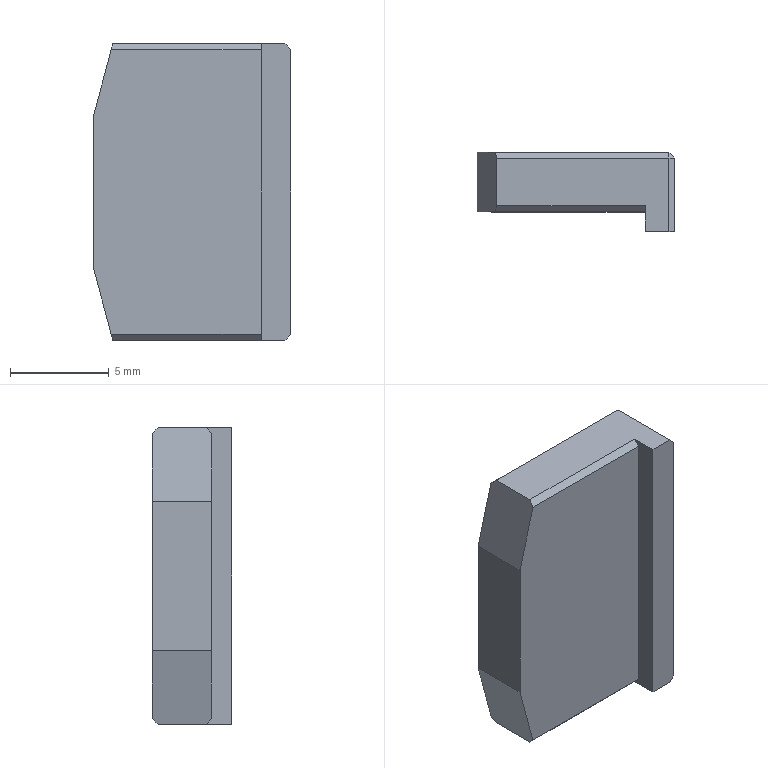Part | STEP file | Brake block | 1 solid | 25 faces | box 10 x 4 x 15 mm | volume 442.73 mm3 | plane 21 | cylinder 4 | commonest cylinder face diameters 3.2 x4